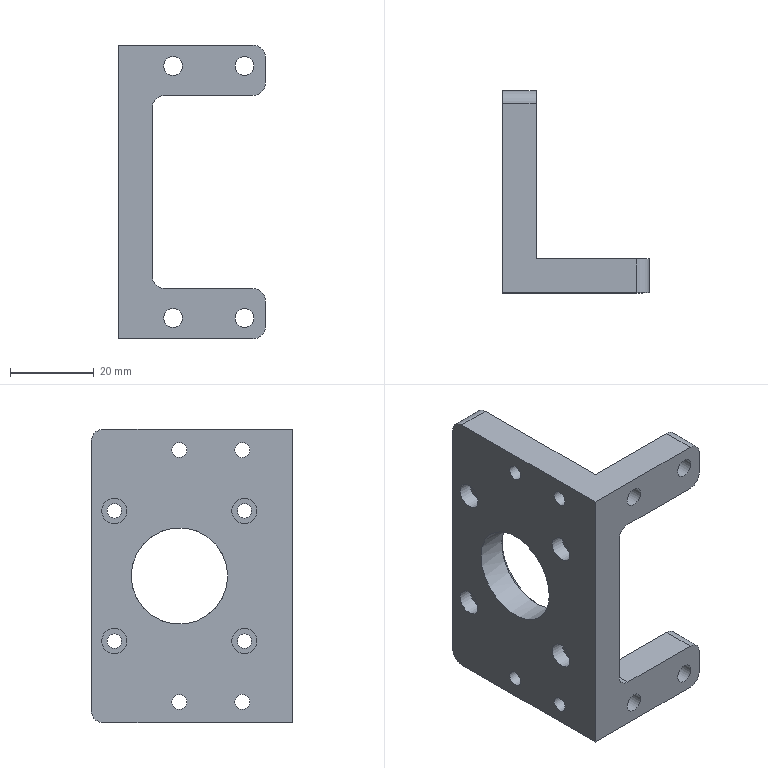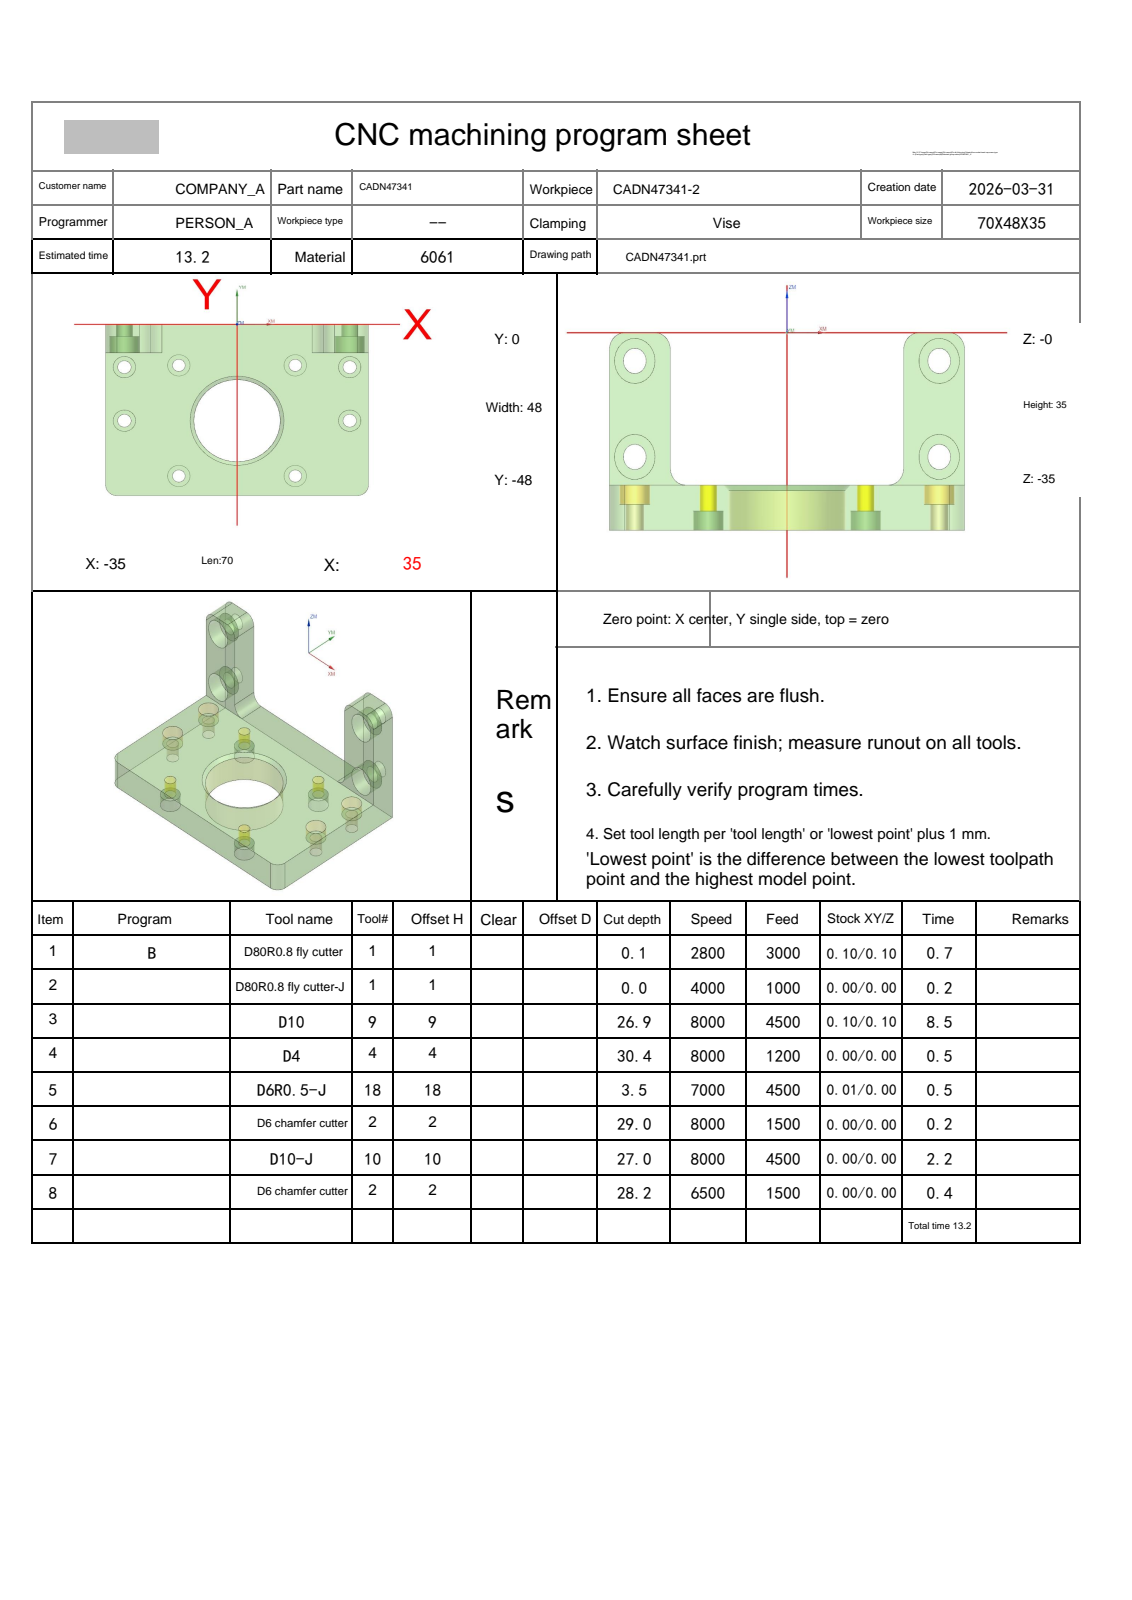NC program | NX | posted by the shop | part box 35 x 48 x 70 mm
Lines 111 to 1256 of 13995:
N3 T09 M06
(D10  D=10. R=0. H=09 ce=0.10 di=0.10)
G00 G90 G54 X7. Y-62.5 M03 S8000
G43 H09 Z14.5
M08
Z.702
G01 Z-.498 F4500.
Y-55.078
G03 X0.0 Y-48.078 I-7. J0.0
G01 X-32.615
X-32.647 Y-48.071
X-33.025 Y-47.905
X-33.221 Y-47.868
X-33.251 Y-47.856
X-34.152 Y-47.253
X-34.172 Y-47.234
X-34.785 Y-46.394
X-34.798 Y-46.365
X-34.837 Y-46.198
X-34.878 Y-46.096
X-35.063 Y-45.721
X-35.071 Y-45.686
X-35.08 Y-44.298
Y-13.178
G02 X-40.18 Y-8. I.185 J5.282
G01 Y0.0
X-40.185 Y.085
X-40.1 Y.08
X-38.831
Y0.0
Y-.08
Y-8.
G03 X-33.693 Y-13.1 I5.137 J.037
G01 X-33.656
X-24.344
X-24.307
G03 X-19.169 Y-8. I0.0 J5.137
G01 Y-.003
Y.08
X19.169
Y0.0
Y-.08
Y-8.
G03 X24.307 Y-13.1 I5.137 J.037
G01 X24.344
X33.656
X33.693
G03 X38.831 Y-8. I0.0 J5.137
G01 Y-.003
Y.079
X39.217
X40.1 Y.08
X40.185 Y.085
X40.18 Y0.0
X40.177 Y-8.115
G02 X35.08 Y-13.178 I-5.226 J.163
G01 Y-44.298
X35.071 Y-45.749
X35.06 Y-45.79
X34.877 Y-46.098
X34.837 Y-46.198
X34.744 Y-46.594
X34.722 Y-46.633
X33.914 Y-47.413
X33.251 Y-47.856
X33.223 Y-47.868
X33.003 Y-47.913
X32.647 Y-48.071
X32.615 Y-48.078
X3.014
G02 X2.201 Y-47.66 I0.0 J1.
G01 X-2.201 Y-41.496
G03 X-3.014 Y-41.078 I-.813 J-.582
G01 X-27.081
G02 X-28.08 Y-40.079 I.001 J1.
G01 Y-21.099
G02 X-27.081 Y-20.1 I1. J-.001
G01 X-24.364
X-24.307
G03 X-13.732 Y-13.92 I0.0 J12.137
X-12.169 Y-7.963 I-10.575 J5.957
G01 Y-7.919
G02 X-11.171 Y-6.92 I1. J-.001
G01 X11.171
G02 X12.169 Y-7.919 I-.001 J-1.
G01 Y-8.025
G03 X24.307 Y-20.1 I12.137 J.062
G01 X24.364
X27.081
G02 X28.08 Y-21.099 I-.001 J-1.
G01 Y-40.079
G02 X27.081 Y-41.078 I-1. J.001
G01 X3.014
G02 X2.201 Y-40.66 I0.0 J1.
G01 X-2.201 Y-34.496
G03 X-3.014 Y-34.078 I-.814 J-.582
G01 X-12.866
G02 X-13.56 Y-33.798 I0.0 J1.
G01 X-14.979 Y-32.43
G03 X-15.458 Y-32.174 I-.694 J-.72
G02 X-17.421 Y-29.732 I.536 J2.442
X-15.603 Y-27.327 I2.5 J0.0
G01 X-8.066 Y-25.191
G02 X-7.384 Y-25.097 I.682 J-2.405
X-4.884 Y-27.597 I0.0 J-2.5
X-6.703 Y-30.002 I-2.5 J0.0
G01 X-13.018 Y-31.791
G03 X-13.502 Y-32.1 I.273 J-.962
G01 X-14.911 Y-33.732
G02 X-15.667 Y-34.078 I-.757 J.654
G01 X-20.082
G02 X-21.08 Y-33.08 I.002 J1.
G01 Y-27.65
G02 X-20.292 Y-26.674 I1. J-.002
G03 X-6.347 Y-14.573 I-4.015 J18.711
G02 X-5.411 Y-13.92 I.938 J-.347
G01 X5.411
G02 X6.347 Y-14.573 I-.002 J-1.
G03 X20.292 Y-26.674 I17.959 J6.61
G02 X21.08 Y-27.65 I-.212 J-.977
G01 Y-33.08
G02 X20.082 Y-34.078 I-1. J.002
G01 X15.668
G02 X14.911 Y-33.732 I0.0 J1.
G01 X13.502 Y-32.1
G03 X13.018 Y-31.791 I-.757 J-.654
G01 X6.703 Y-30.002
G02 X4.884 Y-27.597 I.682 J2.405
X7.384 Y-25.097 I2.5 J0.0
X8.066 Y-25.191 I0.0 J-2.5
G01 X15.603 Y-27.327
G02 X17.421 Y-29.732 I-.682 J-2.405
X15.458 Y-32.174 I-2.5 J0.0
G03 X14.979 Y-32.431 I.215 J-.977
G01 X13.56 Y-33.798
G02 X12.866 Y-34.078 I-.694 J.72
G01 X3.014
G02 X2.201 Y-33.66 I0.0 J1.
G01 X-2.201 Y-27.496
G03 X-3.014 Y-27.078 I-.814 J-.582
G01 X-4.103
G02 X-5.101 Y-26.078 I.002 J1.
X-4.847 Y-25.412 I1. J0.0
G03 X-1.89 Y-21.404 I-19.46 J17.449
G02 X-1.036 Y-20.92 I.857 J-.516
G01 X1.036
G02 X1.89 Y-21.404 I-.002 J-1.
G03 X4.847 Y-25.412 I22.416 J13.441
G02 X5.101 Y-26.078 I-.746 J-.666
X4.103 Y-27.078 I-1. J0.0
G01 X0.0
X-.5
G03 X-7.5 Y-34.078 I0.0 J-7.
G01 Z.702
G00 Z3.
G01 X7. Y-62.5 F6000.
G00 Z.204
G01 Z-.996 F4500.
Y-55.078
G03 X0.0 Y-48.078 I-7. J0.0
G01 X-32.615
X-32.647 Y-48.071
X-33.025 Y-47.905
X-33.221 Y-47.868
X-33.251 Y-47.856
X-34.152 Y-47.253
X-34.172 Y-47.234
X-34.785 Y-46.394
X-34.798 Y-46.365
X-34.837 Y-46.198
X-34.878 Y-46.096
X-35.063 Y-45.721
X-35.071 Y-45.686
X-35.08 Y-44.298
Y-13.178
G02 X-40.18 Y-8. I.185 J5.282
G01 Y0.0
X-40.185 Y.085
X-40.1 Y.08
X-39.365
Y-.08
Y-8.
G03 X-34.249 Y-13.1 I5.116 J.016
G01 X-34.233
X-23.767
X-23.751
G03 X-18.635 Y-8. I0.0 J5.116
G01 Y-.009
Y.08
X18.635
Y0.0
Y-.08
Y-8.
G03 X23.751 Y-13.1 I5.116 J.016
G01 X23.767
X34.233
X34.249
G03 X39.365 Y-8. I0.0 J5.116
G01 Y-.08
Y0.0
Y.08
X40.1
X40.185 Y.085
X40.18 Y0.0
X40.177 Y-8.115
G02 X35.08 Y-13.178 I-5.226 J.163
G01 Y-44.298
X35.071 Y-45.749
X35.06 Y-45.79
X34.877 Y-46.098
X34.837 Y-46.198
X34.744 Y-46.594
X34.722 Y-46.633
X33.914 Y-47.413
X33.251 Y-47.856
X33.223 Y-47.868
X33.003 Y-47.913
X32.647 Y-48.071
X32.615 Y-48.078
X3.014
G02 X2.201 Y-47.66 I0.0 J1.
G01 X-2.201 Y-41.496
G03 X-3.014 Y-41.078 I-.813 J-.582
G01 X-27.082
G02 X-28.08 Y-40.08 I.002 J1.
G01 Y-21.098
G02 X-27.082 Y-20.1 I1. J-.002
G01 X-23.776
X-23.751
G03 X-13.189 Y-13.92 I0.0 J12.116
X-11.634 Y-7.983 I-10.562 J5.937
G01 X-11.635 Y-7.919
G02 X-10.636 Y-6.92 I1. J-.002
G01 X10.636
G02 X11.635 Y-7.919 I-.002 J-1.
G01 Y-8.011
G03 X23.751 Y-20.1 I12.116 J.028
G01 X23.776
X27.082
G02 X28.08 Y-21.098 I-.002 J-1.
G01 Y-40.08
G02 X27.082 Y-41.078 I-1. J.002
G01 X3.014
G02 X2.201 Y-40.66 I0.0 J1.
G01 X-2.201 Y-34.496
G03 X-3.014 Y-34.078 I-.814 J-.582
G01 X-12.316
G02 X-13.01 Y-33.798 I0.0 J1.
G01 X-14.428 Y-32.431
G03 X-14.907 Y-32.174 I-.694 J-.72
G02 X-16.871 Y-29.732 I.536 J2.442
X-15.053 Y-27.327 I2.5 J0.0
G01 X-7.52 Y-25.192
G02 X-6.838 Y-25.097 I.682 J-2.405
X-4.338 Y-27.597 I0.0 J-2.5
X-6.156 Y-30.003 I-2.5 J0.0
G01 X-12.468 Y-31.791
G03 X-12.952 Y-32.1 I.273 J-.962
G01 X-14.361 Y-33.732
G02 X-15.117 Y-34.078 I-.757 J.654
G01 X-20.082
G02 X-21.08 Y-33.08 I.002 J1.
G01 Y-27.76
G02 X-20.264 Y-26.779 I1. J-.002
G03 X-5.806 Y-14.574 I-3.487 J18.796
G02 X-4.87 Y-13.92 I.938 J-.347
G01 X4.87
G02 X5.806 Y-14.574 I-.002 J-1.
G03 X20.264 Y-26.779 I17.945 J6.59
G02 X21.08 Y-27.76 I-.184 J-.983
G01 Y-33.08
G02 X20.082 Y-34.078 I-1. J.002
G01 X15.117
G02 X14.36 Y-33.731 I0.0 J1.
G01 X12.952 Y-32.1
G03 X12.468 Y-31.791 I-.757 J-.653
G01 X6.156 Y-30.003
G02 X4.338 Y-27.597 I.682 J2.405
X6.838 Y-25.097 I2.5 J0.0
X7.52 Y-25.192 I0.0 J-2.5
G01 X15.053 Y-27.327
G02 X16.871 Y-29.732 I-.682 J-2.405
X14.908 Y-32.174 I-2.5 J0.0
G03 X14.428 Y-32.431 I.215 J-.977
G01 X13.01 Y-33.798
G02 X12.316 Y-34.078 I-.694 J.72
G01 X3.014
G02 X2.201 Y-33.66 I0.0 J1.
G01 X-2.201 Y-27.496
G03 X-3.014 Y-27.078 I-.814 J-.582
G01 X-3.557
G02 X-4.555 Y-26.078 I.002 J1.
X-4.301 Y-25.412 I1. J0.0
G03 X-1.347 Y-21.404 I-19.45 J17.429
G02 X-.492 Y-20.92 I.857 J-.516
G01 X.492
G02 X1.347 Y-21.404 I-.002 J-1.
G03 X4.301 Y-25.412 I22.404 J13.421
G02 X4.555 Y-26.078 I-.746 J-.666
X3.557 Y-27.078 I-1. J0.0
G01 X0.0
X-.5
G03 X-7.5 Y-34.078 I0.0 J-7.
G01 Z.204
G00 Z3.
G01 X7. Y-62.5 F6000.
G00 Z-.294
G01 Z-1.494 F4500.
Y-55.078
G03 X0.0 Y-48.078 I-7. J0.0
G01 X-32.615
X-32.647 Y-48.071
X-33.025 Y-47.905
X-33.221 Y-47.868
X-33.251 Y-47.856
X-34.152 Y-47.253
X-34.172 Y-47.234
X-34.785 Y-46.394
X-34.798 Y-46.365
X-34.837 Y-46.198
X-34.878 Y-46.096
X-35.063 Y-45.721
X-35.071 Y-45.686
X-35.08 Y-44.298
Y-13.178
G02 X-40.18 Y-8. I.185 J5.282
G01 Y0.0
X-40.185 Y.085
X-40.1 Y.08
X-39.71
Y-.08
Y-8.
G03 X-34.603 Y-13.1 I5.107 J.007
G01 X-34.595
X-23.405
X-23.397
G03 X-18.29 Y-8. I0.0 J5.107
G01 Y-.006
Y.08
X18.29
Y-.08
Y-8.
G03 X23.397 Y-13.1 I5.107 J.007
G01 X23.405
X34.595
X34.603
G03 X39.71 Y-8. I0.0 J5.107
G01 Y-.08
Y0.0
Y.08
X40.1
X40.185 Y.085
X40.18 Y0.0
X40.177 Y-8.115
G02 X35.08 Y-13.178 I-5.226 J.163
G01 Y-44.298
X35.071 Y-45.749
X35.06 Y-45.79
X34.877 Y-46.098
X34.837 Y-46.198
X34.744 Y-46.594
X34.722 Y-46.633
X33.914 Y-47.413
X33.251 Y-47.856
X33.223 Y-47.868
X33.003 Y-47.913
X32.647 Y-48.071
X32.615 Y-48.078
X3.014
G02 X2.201 Y-47.66 I0.0 J1.
G01 X-2.201 Y-41.496
G03 X-3.014 Y-41.078 I-.813 J-.582
G01 X-27.082
G02 X-28.08 Y-40.08 I.002 J1.
G01 Y-21.098
G02 X-27.082 Y-20.1 I1. J-.002
G01 X-23.409
X-23.397
G03 X-12.84 Y-13.92 I0.0 J12.107
X-11.29 Y-7.992 I-10.557 J5.928
G01 Y-7.918
G02 X-10.292 Y-6.92 I1. J-.002
G01 X10.292
G02 X11.293 Y-7.924 I-.002 J-1.004
G01 X11.29 Y-8.005
G03 X23.397 Y-20.1 I12.107 J.012
G01 X23.409
X27.082
G02 X28.08 Y-21.098 I-.002 J-1.
G01 Y-40.08
G02 X27.082 Y-41.078 I-1. J.002
G01 X3.014
G02 X2.201 Y-40.66 I0.0 J1.
G01 X-2.201 Y-34.496
G03 X-3.014 Y-34.078 I-.814 J-.582
G01 X-11.965
G02 X-12.659 Y-33.798 I0.0 J1.
G01 X-14.077 Y-32.431
G03 X-14.556 Y-32.174 I-.694 J-.72
G02 X-16.52 Y-29.733 I.536 J2.442
X-14.702 Y-27.327 I2.5 J0.0
G01 X-7.17 Y-25.192
G02 X-6.488 Y-25.098 I.682 J-2.405
X-3.988 Y-27.598 I0.0 J-2.5
X-5.807 Y-30.003 I-2.5 J0.0
G01 X-12.117 Y-31.791
G03 X-12.601 Y-32.1 I.273 J-.962
G01 X-14.009 Y-33.732
G02 X-14.766 Y-34.078 I-.757 J.654
G01 X-20.082
G02 X-21.08 Y-33.08 I.002 J1.
G01 Y-27.822
G02 X-20.247 Y-26.838 I1. J-.002
G03 X-5.459 Y-14.574 I-3.15 J18.846
G02 X-4.523 Y-13.92 I.938 J-.347
G01 X4.523
G02 X5.459 Y-14.574 I-.002 J-1.
G03 X20.247 Y-26.838 I17.938 J6.581
G02 X21.08 Y-27.822 I-.167 J-.986
G01 Y-33.08
G02 X20.082 Y-34.078 I-1. J.002
G01 X14.766
G02 X14.009 Y-33.731 I0.0 J1.
G01 X12.601 Y-32.1
G03 X12.117 Y-31.791 I-.757 J-.653
G01 X5.807 Y-30.003
G02 X3.988 Y-27.598 I.682 J2.405
X6.488 Y-25.098 I2.5 J0.0
X7.17 Y-25.192 I0.0 J-2.5
G01 X14.702 Y-27.327
G02 X16.52 Y-29.733 I-.682 J-2.405
X14.556 Y-32.174 I-2.5 J0.0
G03 X14.077 Y-32.431 I.215 J-.977
G01 X12.659 Y-33.798
G02 X11.965 Y-34.078 I-.694 J.72
G01 X3.014
G02 X2.201 Y-33.66 I0.0 J1.
G01 X-2.201 Y-27.496
G03 X-3.014 Y-27.078 I-.814 J-.582
G01 X-3.208
G02 X-4.205 Y-26.078 I.002 J1.
X-3.952 Y-25.413 I1. J0.0
G03 X-.998 Y-21.404 I-19.446 J17.42
G02 X-.144 Y-20.92 I.857 J-.516
G01 X.144
G02 X.998 Y-21.404 I-.002 J-1.
G03 X3.952 Y-25.413 I22.399 J13.412
G02 X4.205 Y-26.078 I-.746 J-.665
X3.208 Y-27.078 I-1. J0.0
G01 X0.0
X-.5
G03 X-7.5 Y-34.078 I0.0 J-7.
G01 Z-.294
G00 Z3.
G01 X7. Y-62.5 F6000.
G00 Z-.793
G01 Z-1.993 F4500.
Y-55.078
G03 X0.0 Y-48.078 I-7. J0.0
G01 X-32.615
X-32.647 Y-48.071
X-33.025 Y-47.905
X-33.221 Y-47.868
X-33.251 Y-47.856
X-34.152 Y-47.253
X-34.172 Y-47.234
X-34.785 Y-46.394
X-34.798 Y-46.365
X-34.837 Y-46.198
X-34.878 Y-46.096
X-35.063 Y-45.721
X-35.071 Y-45.686
X-35.08 Y-44.298
Y-13.178
G02 X-40.18 Y-8. I.185 J5.282
G01 Y0.0
X-40.185 Y.085
X-40.1 Y.08
X-39.932
Y-.08
Y-8.
G03 X-34.826 Y-13.1 I5.123 J.023
G01 X-23.174
G03 X-18.068 Y-8. I-.008 J5.114
G01 Y-.003
Y.08
X18.068
Y.003
Y-6.92
Y-8.
G03 X23.174 Y-13.1 I5.119 J.019
G01 X34.826
G03 X39.932 Y-8. I-.017 J5.123
G01 Y-.08
Y0.0
Y.002
Y.08
X40.1
X40.185 Y.085
X40.18 Y0.0
X40.177 Y-8.115
G02 X35.08 Y-13.178 I-5.226 J.163
G01 Y-44.298
X35.071 Y-45.749
X35.06 Y-45.79
X34.877 Y-46.098
X34.837 Y-46.198
X34.744 Y-46.594
X34.722 Y-46.633
X33.914 Y-47.413
X33.251 Y-47.856
X33.223 Y-47.868
X33.003 Y-47.913
X32.647 Y-48.071
X32.615 Y-48.078
X3.014
G02 X2.201 Y-47.66 I0.0 J1.
G01 X-2.201 Y-41.496
G03 X-3.014 Y-41.078 I-.814 J-.582
G01 X-27.082
G02 X-28.08 Y-40.08 I.002 J1.
G01 Y-21.098
G02 X-27.082 Y-20.1 I1. J-.002
G01 X-23.163
G03 X-12.621 Y-13.92 I-.019 J12.114
X-11.068 Y-7.986 I-10.561 J5.934
G01 Y-7.918
G02 X-10.07 Y-6.92 I1. J-.002
G01 X10.07
G02 X11.068 Y-7.918 I-.002 J-1.
G01 Y-8.013
G03 X23.165 Y-20.1 I12.119 J.032
G01 X27.082
G02 X28.08 Y-21.098 I-.002 J-1.
G01 Y-40.08
G02 X27.082 Y-41.078 I-1. J.002
G01 X3.014
G02 X2.201 Y-40.66 I0.0 J1.
G01 X-2.201 Y-34.496
G03 X-3.014 Y-34.078 I-.814 J-.582
G01 X-11.748
G02 X-12.442 Y-33.798 I0.0 J1.
G01 X-13.86 Y-32.431
G03 X-14.339 Y-32.174 I-.694 J-.72
G02 X-16.303 Y-29.732 I.536 J2.442
X-14.485 Y-27.327 I2.5 J0.0
G01 X-6.952 Y-25.192
G02 X-6.27 Y-25.097 I.682 J-2.405
X-3.77 Y-27.597 I0.0 J-2.5
X-5.589 Y-30.003 I-2.5 J0.0
G01 X-11.9 Y-31.791
G03 X-12.384 Y-32.1 I.273 J-.962
G01 X-13.793 Y-33.732
G02 X-14.549 Y-34.078 I-.757 J.654
G01 X-20.082
G02 X-21.08 Y-33.08 I.002 J1.
G01 Y-27.857
G02 X-20.237 Y-26.872 I1. J-.002
G03 X-5.239 Y-14.573 I-2.946 J18.886
G02 X-4.304 Y-13.92 I.938 J-.347
G01 X4.305
G02 X5.241 Y-14.573 I-.002 J-1.
G03 X20.237 Y-26.871 I17.947 J6.592
G02 X21.08 Y-27.856 I-.157 J-.988
G01 Y-33.08
G02 X20.082 Y-34.078 I-1. J.002
G01 X14.553
G02 X13.796 Y-33.731 I0.0 J1.
G01 X12.388 Y-32.1
G03 X11.903 Y-31.791 I-.757 J-.653
G01 X5.591 Y-30.002
G02 X3.773 Y-27.597 I.682 J2.405
X6.273 Y-25.097 I2.5 J0.0
X6.955 Y-25.192 I0.0 J-2.5
G01 X14.489 Y-27.327
G02 X16.307 Y-29.732 I-.682 J-2.405
X14.343 Y-32.174 I-2.5 J0.0
G03 X13.864 Y-32.431 I.215 J-.977
G01 X12.445 Y-33.798
G02 X11.751 Y-34.078 I-.694 J.72
G01 X3.014
G02 X2.201 Y-33.66 I0.0 J1.
G01 X-2.201 Y-27.496
G03 X-3.001 Y-27.078 I-.814 J-.582
G02 X-3.987 Y-26.078 I.014 J1.
X-3.733 Y-25.413 I1. J0.0
G03 X-.853 Y-21.526 I-19.449 J17.427
G02 X.001 Y-21.047 I.854 J-.521
X.855 Y-21.526 I0.0 J-1.
G03 X3.736 Y-25.413 I22.332 J13.545
G02 X3.99 Y-26.078 I-.746 J-.665
X2.992 Y-27.078 I-1. J0.0
G01 X0.0
X-.5
G03 X-7.5 Y-34.078 I0.0 J-7.
G01 Z-.793
G00 Z3.
G01 X7. Y-62.5 F6000.
G00 Z-1.291
G01 Z-2.491 F4500.
Y-55.078
G03 X0.0 Y-48.078 I-7. J0.0
G01 X-32.615
X-32.647 Y-48.071
X-33.025 Y-47.905
X-33.221 Y-47.868
X-33.251 Y-47.856
X-34.152 Y-47.253
X-34.172 Y-47.234
X-34.785 Y-46.394
X-34.798 Y-46.365
X-34.837 Y-46.198
X-34.878 Y-46.096
X-35.063 Y-45.721
X-35.071 Y-45.686
X-35.08 Y-44.298
Y-13.178
G02 X-40.18 Y-8. I.185 J5.282
G01 Y0.0
X-40.196 Y.072
X-40.122 Y.077
X-40.057 Y.076
X-40.058 Y-8.
G03 X-34.957 Y-13.1 I5.14 J.04
G01 X-23.043
G03 X-17.942 Y-8. I-.037 J5.138
G01 Y-6.92
Y.008
Y.009
Y.08
X17.942
Y.009
X17.941 Y.008
X17.942 Y-6.92
Y-8.
G03 X23.043 Y-13.1 I5.1 J0.0
G01 X34.957
G03 X40.058 Y-8. I-.039 J5.14
G01 X40.057 Y.076
X40.122 Y.077
X40.196 Y.072
X40.18 Y0.0
X40.177 Y-8.115
G02 X35.08 Y-13.178 I-5.226 J.163
G01 Y-14.498
Y-44.298
X35.071 Y-45.749
X35.06 Y-45.79
X34.877 Y-46.098
X34.837 Y-46.198
X34.744 Y-46.594
X34.722 Y-46.633
X33.914 Y-47.413
X33.251 Y-47.856
X33.223 Y-47.868
X33.003 Y-47.913
X32.647 Y-48.071
X32.615 Y-48.078
X3.014
G02 X2.201 Y-47.66 I0.0 J1.
G01 X-2.201 Y-41.496
G03 X-3.014 Y-41.078 I-.813 J-.582
G01 X-27.083
G02 X-28.08 Y-40.081 I.003 J1.
G01 Y-21.097
G02 X-27.083 Y-20.1 I1. J-.003
G01 X-22.993
G03 X-12.505 Y-13.92 I-.086 J12.137
X-10.942 Y-7.963 I-10.575 J5.958
G01 Y-7.918
G02 X-9.945 Y-6.92 I1. J-.003
G01 X9.945
G02 X10.942 Y-7.918 I-.003 J-1.
G01 Y-8.
G03 X23.042 Y-20.1 I12.1 J0.0
G01 X23.044
X27.083
G02 X28.08 Y-21.097 I-.003 J-1.
G01 Y-40.081
G02 X27.083 Y-41.078 I-1. J.003
G01 X3.014
G02 X2.201 Y-40.66 I0.0 J1.
G01 X-2.201 Y-34.496
G03 X-3.014 Y-34.078 I-.814 J-.582
G01 X-11.639
G02 X-12.333 Y-33.798 I0.0 J1.
G01 X-13.752 Y-32.43
G03 X-14.231 Y-32.174 I-.694 J-.72
G02 X-16.194 Y-29.732 I.536 J2.442
X-14.376 Y-27.327 I2.5 J0.0
G01 X-6.839 Y-25.191
G02 X-6.157 Y-25.097 I.682 J-2.405
X-3.657 Y-27.597 I0.0 J-2.5
X-5.476 Y-30.002 I-2.5 J0.0
G01 X-11.791 Y-31.791
G03 X-12.275 Y-32.1 I.273 J-.962
G01 X-13.684 Y-33.732
G02 X-14.441 Y-34.078 I-.757 J.654
G01 X-20.083
G02 X-21.08 Y-33.081 I.003 J1.
G01 Y-27.873
G02 X-20.232 Y-26.887 I1. J-.003
G03 X-5.12 Y-14.572 I-2.848 J18.925
G02 X-4.185 Y-13.92 I.937 J-.348
G01 X4.174
G02 X5.109 Y-14.573 I-.003 J-1.
G03 X20.23 Y-26.892 I17.934 J6.574
G02 X21.08 Y-27.878 I-.15 J-.989
G01 Y-33.081
G02 X20.083 Y-34.078 I-1. J.003
G01 X14.413
G02 X13.656 Y-33.731 I0.0 J1.
G01 X12.247 Y-32.1
G03 X11.763 Y-31.791 I-.757 J-.653
G01 X5.454 Y-30.003
G02 X3.636 Y-27.598 I.682 J2.405
X6.136 Y-25.098 I2.5 J0.0
X6.818 Y-25.192 I0.0 J-2.5
G01 X14.349 Y-27.327
G02 X16.167 Y-29.733 I-.682 J-2.405
X14.203 Y-32.174 I-2.5 J0.0
G03 X13.723 Y-32.431 I.214 J-.977
G01 X12.305 Y-33.798
G02 X11.611 Y-34.078 I-.694 J.72
G01 X3.014
G02 X2.201 Y-33.66 I0.0 J1.
G01 X-2.205 Y-27.491
G03 X-2.946 Y-27.075 I-.814 J-.581
G02 X-3.874 Y-26.078 I.072 J.997
X-3.62 Y-25.413 I1. J0.0
G03 X-.857 Y-21.722 I-19.459 J17.45
G02 X-.008 Y-21.251 I.849 J-.529
X.841 Y-21.723 I0.0 J-1.
G03 X3.6 Y-25.413 I22.202 J13.723
G02 X3.853 Y-26.078 I-.747 J-.665
X2.856 Y-27.078 I-1. J0.0
G01 X0.0
X-.5
G03 X-7.5 Y-34.078 I0.0 J-7.
G01 Z-1.291
G00 Z3.
G01 X7. Y-62.5 F6000.
G00 Z-1.789
G01 Z-2.989 F4500.
Y-55.078
G03 X0.0 Y-48.078 I-7. J0.0
G01 X-32.615
X-32.647 Y-48.071
X-33.025 Y-47.905
X-33.221 Y-47.868
X-33.251 Y-47.856
X-34.152 Y-47.253
X-34.172 Y-47.234
X-34.785 Y-46.394
X-34.798 Y-46.365
X-34.837 Y-46.198
X-34.878 Y-46.096
X-35.063 Y-45.721
X-35.071 Y-45.686
X-35.08 Y-44.298
Y-14.5
Y-13.178
G02 X-40.18 Y-8. I.185 J5.282
G01 Y0.0
X-40.191 Y.078
X-40.113 Y.079
X-40.099
X-40.1 Y-8.
G03 X-35. Y-13.1 I5.1 J0.0
G01 X-23.
G03 X-17.9 Y-8. I0.0 J5.1
G01 Y0.0
Y.001
Y.08
X17.9
X17.899 Y-.08
X17.9 Y-8.
G03 X23. Y-13.1 I5.1 J0.0
G01 X35.
G03 X40.1 Y-8. I0.0 J5.1
G01 X40.099 Y.079
X40.112
X40.191 Y.078
X40.18 Y0.0
X40.177 Y-8.115
G02 X38. Y-12.199 I-5.226 J.163
X35.08 Y-13.178 I-3.049 J4.247
G01 Y-14.5
Y-44.298
X35.071 Y-45.749
X35.06 Y-45.79
X34.877 Y-46.098
X34.837 Y-46.198
X34.744 Y-46.594
X34.722 Y-46.633
X33.914 Y-47.413
X33.251 Y-47.856
X33.223 Y-47.868
X33.003 Y-47.913
X32.647 Y-48.071
X32.615 Y-48.078
X3.014
G02 X2.201 Y-47.66 I0.0 J1.
G01 X-2.201 Y-41.496
G03 X-3.014 Y-41.078 I-.814 J-.582
G01 X-27.083
G02 X-28.08 Y-40.081 I.003 J1.
G01 Y-21.097
G02 X-27.083 Y-20.1 I1. J-.003
G01 X-23.
G03 X-12.447 Y-13.92 I0.0 J12.1
X-10.9 Y-7.999 I-10.553 J5.921
G01 Y-7.917
G02 X-9.903 Y-6.92 I1. J-.003
G01 X9.903
G02 X10.9 Y-7.918 I-.003 J-1.
G01 Y-8.
G03 X23. Y-20.1 I12.1 J0.0
G01 X27.083
G02 X28.08 Y-21.097 I-.003 J-1.
G01 Y-40.081
G02 X27.083 Y-41.078 I-1. J.003
G01 X3.014
G02 X2.201 Y-40.66 I0.0 J1.
G01 X-2.201 Y-34.496
G03 X-3.014 Y-34.078 I-.814 J-.582
G01 X-11.569
G02 X-12.263 Y-33.798 I0.0 J1.
G01 X-13.681 Y-32.431
G03 X-14.16 Y-32.174 I-.694 J-.72
G02 X-16.125 Y-29.733 I.536 J2.442
X-14.306 Y-27.327 I2.5 J0.0
G01 X-6.776 Y-25.193
G02 X-6.094 Y-25.098 I.682 J-2.405
X-3.594 Y-27.598 I0.0 J-2.5
X-5.412 Y-30.003 I-2.5 J0.0
G01 X-11.721 Y-31.791
G03 X-12.205 Y-32.1 I.273 J-.962
G01 X-13.614 Y-33.731
G02 X-14.371 Y-34.078 I-.757 J.653
G01 X-20.083
G02 X-21.08 Y-33.081 I.003 J1.
G01 Y-27.884
G02 X-20.228 Y-26.898 I1. J-.003
G03 X-5.067 Y-14.573 I-2.772 J18.898
G02 X-4.127 Y-13.918 I.94 J-.347
G01 X-4.063 Y-13.92
X4.132
G02 X5.066 Y-14.573 I-.003 J-1.
G03 X20.228 Y-26.898 I17.933 J6.573
G02 X21.08 Y-27.884 I-.148 J-.989
G01 Y-33.081
G02 X20.083 Y-34.078 I-1. J.003
G01 X14.37
G02 X13.613 Y-33.731 I0.0 J1.
G01 X12.205 Y-32.1
G03 X11.721 Y-31.791 I-.757 J-.653
G01 X5.412 Y-30.003
G02 X3.594 Y-27.598 I.682 J2.405
X6.094 Y-25.098 I2.5 J0.0
X6.776 Y-25.193 I0.0 J-2.5
G01 X14.306 Y-27.327
G02 X16.124 Y-29.733 I-.682 J-2.405
X14.16 Y-32.174 I-2.5 J0.0
G03 X13.681 Y-32.431 I.214 J-.977
G01 X12.263 Y-33.798
G02 X11.569 Y-34.078 I-.694 J.72
G01 X3.014
G02 X2.201 Y-33.66 I0.0 J1.
G01 X-2.209 Y-27.485
G03 X-2.917 Y-27.072 I-.814 J-.582
G02 X-3.811 Y-26.078 I.106 J.994
X-3.558 Y-25.413 I1. J0.0
G03 X-.847 Y-21.801 I-19.442 J17.413
G02 X0.0 Y-21.332 I.847 J-.531
X.847 Y-21.801 I0.0 J-1.
G03 X3.558 Y-25.413 I22.153 J13.801
G02 X3.811 Y-26.078 I-.747 J-.665
X2.814 Y-27.078 I-1. J0.0
G01 X0.0
X-.5
G03 X-7.5 Y-34.078 I0.0 J-7.
G01 Z-1.789
G00 Z3.
G01 X7. Y-62.5 F6000.
G00 Z-2.287
G01 Z-3.487 F4500.
Y-55.078
G03 X0.0 Y-48.078 I-7. J0.0
G01 X-32.615
X-32.647 Y-48.071
X-33.025 Y-47.905
X-33.221 Y-47.868
X-33.251 Y-47.856
X-34.152 Y-47.253
X-34.172 Y-47.234
X-34.785 Y-46.394
X-34.798 Y-46.365
X-34.837 Y-46.198
X-34.878 Y-46.096
X-35.063 Y-45.721
X-35.071 Y-45.686
X-35.08 Y-44.298
Y-13.178
X-35.188 Y-13.173
X-35.183 Y-13.097
X-35. Y-13.1
X-23.
G03 X-17.9 Y-8. I0.0 J5.1
G01 Y-.003
Y.08
X17.9
Y-.08
Y-8.
G03 X23. Y-13.1 I5.1 J0.0
G01 X35.
X35.162 Y-13.097
X35.165 Y-13.176
X35.08 Y-13.178
Y-44.298
X35.071 Y-45.749
X35.06 Y-45.79
X34.877 Y-46.098
X34.837 Y-46.198
X34.744 Y-46.594
X34.722 Y-46.633
X33.914 Y-47.413
X33.251 Y-47.856
X33.223 Y-47.868
X33.003 Y-47.913
X32.647 Y-48.071
X32.615 Y-48.078
X3.014
G02 X2.201 Y-47.66 I0.0 J1.
G01 X-2.201 Y-41.496
G03 X-3.014 Y-41.078 I-.813 J-.582
G01 X-27.083
G02 X-28.08 Y-40.081 I.003 J1.
G01 Y-21.097
G02 X-27.083 Y-20.1 I1. J-.003
G01 X-23.
G03 X-12.447 Y-13.92 I0.0 J12.1
X-10.9 Y-7.999 I-10.553 J5.921
G01 Y-7.918
G02 X-9.903 Y-6.92 I1. J-.003
G01 X9.903
G02 X10.9 Y-7.918 I-.003 J-1.
G01 Y-8.
G03 X23. Y-20.1 I12.1 J0.0
G01 X27.083
G02 X28.08 Y-21.097 I-.003 J-1.
G01 Y-40.081
G02 X27.083 Y-41.078 I-1. J.003
G01 X3.014
G02 X2.201 Y-40.66 I0.0 J1.
G01 X-2.201 Y-34.496
G03 X-3.014 Y-34.078 I-.814 J-.582
G01 X-11.569
G02 X-12.263 Y-33.798 I0.0 J1.
G01 X-13.681 Y-32.431
G03 X-14.16 Y-32.174 I-.694 J-.72
G02 X-16.124 Y-29.733 I.536 J2.442
X-14.306 Y-27.327 I2.5 J0.0
G01 X-6.776 Y-25.193
G02 X-6.094 Y-25.098 I.682 J-2.405
X-3.594 Y-27.598 I0.0 J-2.5
X-5.412 Y-30.003 I-2.5 J0.0
G01 X-11.721 Y-31.791
G03 X-12.205 Y-32.1 I.273 J-.962
G01 X-13.614 Y-33.731
G02 X-14.37 Y-34.078 I-.757 J.653
G01 X-20.083
G02 X-21.08 Y-33.081 I.003 J1.
G01 Y-27.884
G02 X-20.228 Y-26.898 I1. J-.003
G03 X-5.067 Y-14.573 I-2.772 J18.898
G02 X-4.127 Y-13.918 I.94 J-.347
G01 X-4.063 Y-13.92
X4.131
G02 X5.067 Y-14.573 I-.003 J-1.
G03 X20.228 Y-26.898 I17.933 J6.573
G02 X21.08 Y-27.884 I-.148 J-.989
G01 Y-33.081
G02 X20.083 Y-34.078 I-1. J.003
G01 X14.37
G02 X13.613 Y-33.731 I0.0 J1.
G01 X12.205 Y-32.1
G03 X11.721 Y-31.791 I-.757 J-.653
G01 X5.412 Y-30.003
G02 X3.594 Y-27.598 I.682 J2.405
X6.094 Y-25.098 I2.5 J0.0
X6.776 Y-25.193 I0.0 J-2.5
G01 X14.306 Y-27.327
G02 X16.124 Y-29.733 I-.682 J-2.405
X14.16 Y-32.174 I-2.5 J0.0
G03 X13.681 Y-32.431 I.214 J-.977
G01 X12.263 Y-33.798
G02 X11.569 Y-34.078 I-.694 J.72
G01 X3.014
G02 X2.201 Y-33.66 I0.0 J1.
G01 X-2.209 Y-27.485
G03 X-2.917 Y-27.072 I-.814 J-.582
G02 X-3.811 Y-26.078 I.106 J.994
X-3.558 Y-25.413 I1. J0.0
G03 X-.847 Y-21.801 I-19.442 J17.413
G02 X0.0 Y-21.332 I.847 J-.531
X.847 Y-21.801 I0.0 J-1.
G03 X3.558 Y-25.413 I22.153 J13.801
G02 X3.811 Y-26.078 I-.747 J-.665
X2.814 Y-27.078 I-1. J0.0
G01 X0.0
X-.5
G03 X-7.5 Y-34.078 I0.0 J-7.
G01 Z-2.287
G00 Z3.
G01 X7. Y-62.5 F6000.
G00 Z-2.785
G01 Z-3.985 F4500.
Y-55.078
G03 X0.0 Y-48.078 I-7. J0.0
G01 X-32.615
X-32.647 Y-48.071
X-33.025 Y-47.905
X-33.221 Y-47.868
X-33.251 Y-47.856
X-34.152 Y-47.253
X-34.172 Y-47.234
X-34.785 Y-46.394
X-34.798 Y-46.365
X-34.837 Y-46.198
X-34.878 Y-46.096
X-35.063 Y-45.721
X-35.071 Y-45.686
X-35.08 Y-44.298
Y-13.178
X-35.185 Y-13.173
X-35.181 Y-13.097
X-35. Y-13.1
X-22.998
G03 X-17.9 Y-8. I-.002 J5.1
G01 Y-.003
Y.08
X17.9
Y-.08
Y-8.
G03 X23. Y-13.1 I5.1 J0.0
G01 X35.004
X35.16 Y-13.097
X35.163 Y-13.176
X35.08 Y-13.178
Y-44.298
X35.071 Y-45.749
X35.06 Y-45.79
X34.877 Y-46.098
X34.837 Y-46.198
X34.744 Y-46.594
X34.722 Y-46.633
X33.914 Y-47.413
X33.251 Y-47.856
X33.223 Y-47.868
X33.003 Y-47.913
X32.647 Y-48.071
X32.615 Y-48.078
X3.014
G02 X2.201 Y-47.66 I0.0 J1.
G01 X-2.201 Y-41.496
G03 X-3.014 Y-41.078 I-.813 J-.582
G01 X-27.083
G02 X-28.08 Y-40.081 I.003 J1.
G01 Y-21.097
G02 X-27.083 Y-20.1 I1. J-.003
G01 X-22.996
G03 X-12.447 Y-13.92 I-.004 J12.1
X-10.9 Y-7.999 I-10.553 J5.921
G01 Y-7.917
G02 X-9.903 Y-6.92 I1. J-.003
G01 X9.903
G02 X10.9 Y-7.918 I-.003 J-1.
G01 Y-8.
G03 X22.998 Y-20.1 I12.1 J0.0
G01 X27.083
G02 X28.08 Y-21.097 I-.003 J-1.
G01 Y-40.081
G02 X27.083 Y-41.078 I-1. J.003
G01 X3.014
G02 X2.201 Y-40.66 I0.0 J1.
G01 X-2.201 Y-34.496
G03 X-3.014 Y-34.078 I-.814 J-.582
G01 X-11.569
G02 X-12.263 Y-33.798 I0.0 J1.
G01 X-13.681 Y-32.431
G03 X-14.16 Y-32.175 I-.694 J-.72
G02 X-16.124 Y-29.733 I.536 J2.442
X-14.306 Y-27.327 I2.5 J0.0
G01 X-6.776 Y-25.193
G02 X-6.094 Y-25.098 I.682 J-2.405
X-3.594 Y-27.598 I0.0 J-2.5
X-5.412 Y-30.003 I-2.5 J0.0
G01 X-11.721 Y-31.791
G03 X-12.205 Y-32.1 I.273 J-.962
G01 X-13.614 Y-33.731
G02 X-14.37 Y-34.078 I-.757 J.653
G01 X-20.083
G02 X-21.08 Y-33.081 I.003 J1.
G01 Y-27.884
G02 X-20.228 Y-26.898 I1. J-.003
G03 X-5.067 Y-14.573 I-2.772 J18.898
G02 X-4.127 Y-13.918 I.94 J-.347
G01 X-4.063 Y-13.92
X4.131
G02 X5.066 Y-14.573 I-.003 J-1.
G03 X20.228 Y-26.898 I17.933 J6.573
G02 X21.08 Y-27.884 I-.148 J-.989
G01 Y-33.081
G02 X20.083 Y-34.078 I-1. J.003
G01 X14.37
G02 X13.613 Y-33.731 I0.0 J1.
G01 X12.205 Y-32.1
G03 X11.721 Y-31.791 I-.757 J-.653
G01 X5.412 Y-30.003
G02 X3.594 Y-27.598 I.682 J2.405
X6.094 Y-25.098 I2.5 J0.0
X6.776 Y-25.193 I0.0 J-2.5
G01 X14.306 Y-27.327
G02 X16.124 Y-29.733 I-.682 J-2.405
X14.16 Y-32.174 I-2.5 J0.0
G03 X13.681 Y-32.431 I.214 J-.977
G01 X12.263 Y-33.798
G02 X11.569 Y-34.078 I-.694 J.72
G01 X3.014
G02 X2.201 Y-33.66 I0.0 J1.
G01 X-2.209 Y-27.485
G03 X-2.917 Y-27.072 I-.814 J-.582
G02 X-3.811 Y-26.078 I.106 J.994
X-3.558 Y-25.413 I1. J0.0
G03 X-.847 Y-21.801 I-19.442 J17.413
G02 X0.0 Y-21.332 I.847 J-.531
X.847 Y-21.801 I0.0 J-1.
G03 X3.558 Y-25.413 I22.153 J13.801
G02 X3.811 Y-26.078 I-.747 J-.665
X2.814 Y-27.078 I-1. J0.0
G01 X0.0
X-.5
G03 X-7.5 Y-34.078 I0.0 J-7.
G01 Z-2.785
G00 Z3.